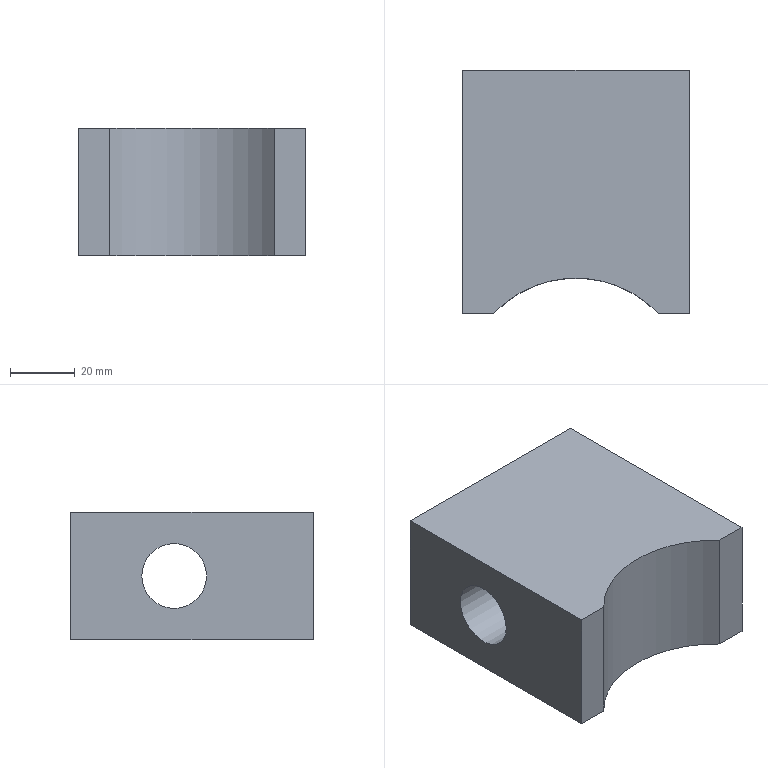Part | NX | features 推移千斤顶约束块 2 | 1 solid | 9 faces | box 70 x 75 x 39.28 mm | volume 169219 mm3 | plane 7 | cylinder 2 | commonest cylinder face diameters 20 x1 70 x1
STEP:
#1=CARTESIAN_POINT('',(0.,-42.,19.64));
#2=VERTEX_POINT('',#1);
#3=CARTESIAN_POINT('',(0.,-32.,19.64));
#4=DIRECTION('',(-1.,0.,0.));
#5=DIRECTION('',(0.,-1.,0.));
#6=AXIS2_PLACEMENT_3D('',#3,#4,#5);
#7=CIRCLE('',#6,10.);
#8=EDGE_CURVE('',#2,#2,#7,.T.);
#9=ORIENTED_EDGE('',*,*,#8,.F.);
#10=EDGE_LOOP('',(#9));
#11=FACE_BOUND('',#10,.T.);
#12=CARTESIAN_POINT('',(0.,0.,0.));
#13=VERTEX_POINT('',#12);
#14=CARTESIAN_POINT('',(0.,-75.,0.));
#15=VERTEX_POINT('',#14);
#16=CARTESIAN_POINT('',(0.,0.,0.));
#17=DIRECTION('',(0.,-1.,0.));
#18=VECTOR('',#17,1000.);
#19=LINE('',#16,#18);
#20=EDGE_CURVE('',#13,#15,#19,.T.);
#21=ORIENTED_EDGE('',*,*,#20,.T.);
#22=CARTESIAN_POINT('',(0.,-75.,39.28));
#23=VERTEX_POINT('',#22);
#24=CARTESIAN_POINT('',(0.,-75.,39.28));
#25=DIRECTION('',(0.,0.,-1.));
#26=VECTOR('',#25,1000.);
#27=LINE('',#24,#26);
#28=EDGE_CURVE('',#23,#15,#27,.T.);
#29=ORIENTED_EDGE('',*,*,#28,.F.);
#30=CARTESIAN_POINT('',(0.,0.,39.28));
#31=VERTEX_POINT('',#30);
#32=CARTESIAN_POINT('',(0.,0.,39.28));
#33=DIRECTION('',(0.,-1.,0.));
#34=VECTOR('',#33,1000.);
#35=LINE('',#32,#34);
#36=EDGE_CURVE('',#31,#23,#35,.T.);
#37=ORIENTED_EDGE('',*,*,#36,.F.);
#38=CARTESIAN_POINT('',(0.,0.,39.28));
#39=DIRECTION('',(0.,0.,-1.));
#40=VECTOR('',#39,1000.);
#41=LINE('',#38,#40);
#42=EDGE_CURVE('',#31,#13,#41,.T.);
#43=ORIENTED_EDGE('',*,*,#42,.T.);
#44=EDGE_LOOP('',(#21,#29,#37,#43));
#45=FACE_BOUND('',#44,.T.);
#46=CARTESIAN_POINT('',(0.,0.,39.28));
#47=DIRECTION('',(1.,0.,0.));
#48=DIRECTION('',(0.,1.,0.));
#49=AXIS2_PLACEMENT_3D('',#46,#47,#48);
#50=PLANE('',#49);
#51=ADVANCED_FACE('',(#11,#45),#50,.F.);
#52=CARTESIAN_POINT('',(9.619,-75.,0.));
#53=VERTEX_POINT('',#52);
#54=CARTESIAN_POINT('',(0.,-75.,0.));
#55=DIRECTION('',(1.,0.,0.));
#56=VECTOR('',#55,1000.);
#57=LINE('',#54,#56);
#58=EDGE_CURVE('',#15,#53,#57,.T.);
#59=ORIENTED_EDGE('',*,*,#58,.T.);
#60=CARTESIAN_POINT('',(9.619,-75.,39.28));
#61=VERTEX_POINT('',#60);
#62=CARTESIAN_POINT('',(9.619,-75.,39.28));
#63=DIRECTION('',(0.,0.,-1.));
#64=VECTOR('',#63,1000.);
#65=LINE('',#62,#64);
#66=EDGE_CURVE('',#61,#53,#65,.T.);
#67=ORIENTED_EDGE('',*,*,#66,.F.);
#68=CARTESIAN_POINT('',(0.,-75.,39.28));
#69=DIRECTION('',(1.,0.,0.));
#70=VECTOR('',#69,1000.);
#71=LINE('',#68,#70);
#72=EDGE_CURVE('',#23,#61,#71,.T.);
#73=ORIENTED_EDGE('',*,*,#72,.F.);
#74=ORIENTED_EDGE('',*,*,#28,.T.);
#75=EDGE_LOOP('',(#59,#67,#73,#74));
#76=FACE_BOUND('',#75,.T.);
#77=CARTESIAN_POINT('',(0.,-75.,39.28));
#78=DIRECTION('',(0.,1.,0.));
#79=DIRECTION('',(-1.,0.,0.));
#80=AXIS2_PLACEMENT_3D('',#77,#78,#79);
#81=PLANE('',#80);
#82=ADVANCED_FACE('',(#76),#81,.F.);
#83=CARTESIAN_POINT('',(60.381,-75.,0.));
#84=VERTEX_POINT('',#83);
#85=CARTESIAN_POINT('',(35.,-99.1,0.));
#86=DIRECTION('',(0.,0.,-1.));
#87=DIRECTION('',(1.,0.,0.));
#88=AXIS2_PLACEMENT_3D('',#85,#86,#87);
#89=CIRCLE('',#88,35.);
#90=EDGE_CURVE('',#53,#84,#89,.T.);
#91=ORIENTED_EDGE('',*,*,#90,.T.);
#92=CARTESIAN_POINT('',(60.381,-75.,39.28));
#93=VERTEX_POINT('',#92);
#94=CARTESIAN_POINT('',(60.381,-75.,39.28));
#95=DIRECTION('',(0.,0.,-1.));
#96=VECTOR('',#95,1000.);
#97=LINE('',#94,#96);
#98=EDGE_CURVE('',#93,#84,#97,.T.);
#99=ORIENTED_EDGE('',*,*,#98,.F.);
#100=CARTESIAN_POINT('',(35.,-99.1,39.28));
#101=DIRECTION('',(0.,0.,-1.));
#102=DIRECTION('',(1.,0.,0.));
#103=AXIS2_PLACEMENT_3D('',#100,#101,#102);
#104=CIRCLE('',#103,35.);
#105=EDGE_CURVE('',#61,#93,#104,.T.);
#106=ORIENTED_EDGE('',*,*,#105,.F.);
#107=ORIENTED_EDGE('',*,*,#66,.T.);
#108=EDGE_LOOP('',(#91,#99,#106,#107));
#109=FACE_BOUND('',#108,.T.);
#110=CARTESIAN_POINT('',(35.,-99.1,39.28));
#111=DIRECTION('',(0.,0.,-1.));
#112=DIRECTION('',(-1.,0.,0.));
#113=AXIS2_PLACEMENT_3D('',#110,#111,#112);
#114=CYLINDRICAL_SURFACE('',#113,35.);
#115=ADVANCED_FACE('',(#109),#114,.F.);
#116=CARTESIAN_POINT('',(70.,-75.,0.));
#117=VERTEX_POINT('',#116);
#118=CARTESIAN_POINT('',(60.381,-75.,0.));
#119=DIRECTION('',(1.,0.,0.));
#120=VECTOR('',#119,1000.);
#121=LINE('',#118,#120);
#122=EDGE_CURVE('',#84,#117,#121,.T.);
#123=ORIENTED_EDGE('',*,*,#122,.T.);
#124=CARTESIAN_POINT('',(70.,-75.,39.28));
#125=VERTEX_POINT('',#124);
#126=CARTESIAN_POINT('',(70.,-75.,39.28));
#127=DIRECTION('',(0.,0.,-1.));
#128=VECTOR('',#127,1000.);
#129=LINE('',#126,#128);
#130=EDGE_CURVE('',#125,#117,#129,.T.);
#131=ORIENTED_EDGE('',*,*,#130,.F.);
#132=CARTESIAN_POINT('',(60.381,-75.,39.28));
#133=DIRECTION('',(1.,0.,0.));
#134=VECTOR('',#133,1000.);
#135=LINE('',#132,#134);
#136=EDGE_CURVE('',#93,#125,#135,.T.);
#137=ORIENTED_EDGE('',*,*,#136,.F.);
#138=ORIENTED_EDGE('',*,*,#98,.T.);
#139=EDGE_LOOP('',(#123,#131,#137,#138));
#140=FACE_BOUND('',#139,.T.);
#141=CARTESIAN_POINT('',(60.381,-75.,39.28));
#142=DIRECTION('',(0.,1.,0.));
#143=DIRECTION('',(0.,0.,1.));
#144=AXIS2_PLACEMENT_3D('',#141,#142,#143);
#145=PLANE('',#144);
#146=ADVANCED_FACE('',(#140),#145,.F.);
#147=CARTESIAN_POINT('',(70.,-42.,19.64));
#148=VERTEX_POINT('',#147);
#149=CARTESIAN_POINT('',(70.,-32.,19.64));
#150=DIRECTION('',(-1.,0.,0.));
#151=DIRECTION('',(0.,-1.,0.));
#152=AXIS2_PLACEMENT_3D('',#149,#150,#151);
#153=CIRCLE('',#152,10.);
#154=EDGE_CURVE('',#148,#148,#153,.T.);
#155=ORIENTED_EDGE('',*,*,#154,.T.);
#156=EDGE_LOOP('',(#155));
#157=FACE_BOUND('',#156,.T.);
#158=CARTESIAN_POINT('',(70.,0.,0.));
#159=VERTEX_POINT('',#158);
#160=CARTESIAN_POINT('',(70.,0.,0.));
#161=DIRECTION('',(0.,1.,0.));
#162=VECTOR('',#161,1000.);
#163=LINE('',#160,#162);
#164=EDGE_CURVE('',#117,#159,#163,.T.);
#165=ORIENTED_EDGE('',*,*,#164,.T.);
#166=CARTESIAN_POINT('',(70.,0.,39.28));
#167=VERTEX_POINT('',#166);
#168=CARTESIAN_POINT('',(70.,0.,39.28));
#169=DIRECTION('',(0.,0.,-1.));
#170=VECTOR('',#169,1000.);
#171=LINE('',#168,#170);
#172=EDGE_CURVE('',#167,#159,#171,.T.);
#173=ORIENTED_EDGE('',*,*,#172,.F.);
#174=CARTESIAN_POINT('',(70.,0.,39.28));
#175=DIRECTION('',(0.,1.,0.));
#176=VECTOR('',#175,1000.);
#177=LINE('',#174,#176);
#178=EDGE_CURVE('',#125,#167,#177,.T.);
#179=ORIENTED_EDGE('',*,*,#178,.F.);
#180=ORIENTED_EDGE('',*,*,#130,.T.);
#181=EDGE_LOOP('',(#165,#173,#179,#180));
#182=FACE_BOUND('',#181,.T.);
#183=CARTESIAN_POINT('',(70.,0.,39.28));
#184=DIRECTION('',(-1.,0.,0.));
#185=DIRECTION('',(0.,-1.,0.));
#186=AXIS2_PLACEMENT_3D('',#183,#184,#185);
#187=PLANE('',#186);
#188=ADVANCED_FACE('',(#157,#182),#187,.F.);
#189=CARTESIAN_POINT('',(0.,0.,0.));
#190=DIRECTION('',(-1.,0.,0.));
#191=VECTOR('',#190,1000.);
#192=LINE('',#189,#191);
#193=EDGE_CURVE('',#159,#13,#192,.T.);
#194=ORIENTED_EDGE('',*,*,#193,.T.);
#195=ORIENTED_EDGE('',*,*,#42,.F.);
#196=CARTESIAN_POINT('',(0.,0.,39.28));
#197=DIRECTION('',(-1.,0.,0.));
#198=VECTOR('',#197,1000.);
#199=LINE('',#196,#198);
#200=EDGE_CURVE('',#167,#31,#199,.T.);
#201=ORIENTED_EDGE('',*,*,#200,.F.);
#202=ORIENTED_EDGE('',*,*,#172,.T.);
#203=EDGE_LOOP('',(#194,#195,#201,#202));
#204=FACE_BOUND('',#203,.T.);
#205=CARTESIAN_POINT('',(0.,0.,39.28));
#206=DIRECTION('',(0.,-1.,0.));
#207=DIRECTION('',(0.,0.,-1.));
#208=AXIS2_PLACEMENT_3D('',#205,#206,#207);
#209=PLANE('',#208);
#210=ADVANCED_FACE('',(#204),#209,.F.);
#211=ORIENTED_EDGE('',*,*,#36,.T.);
#212=ORIENTED_EDGE('',*,*,#72,.T.);
#213=ORIENTED_EDGE('',*,*,#105,.T.);
#214=ORIENTED_EDGE('',*,*,#136,.T.);
#215=ORIENTED_EDGE('',*,*,#178,.T.);
#216=ORIENTED_EDGE('',*,*,#200,.T.);
#217=EDGE_LOOP('',(#211,#212,#213,#214,#215,#216));
#218=FACE_BOUND('',#217,.T.);
#219=CARTESIAN_POINT('',(35.,-99.1,39.28));
#220=DIRECTION('',(0.,0.,1.));
#221=DIRECTION('',(1.,0.,0.));
#222=AXIS2_PLACEMENT_3D('',#219,#220,#221);
#223=PLANE('',#222);
#224=ADVANCED_FACE('',(#218),#223,.T.);
#225=ORIENTED_EDGE('',*,*,#20,.F.);
#226=ORIENTED_EDGE('',*,*,#193,.F.);
#227=ORIENTED_EDGE('',*,*,#164,.F.);
#228=ORIENTED_EDGE('',*,*,#122,.F.);
#229=ORIENTED_EDGE('',*,*,#90,.F.);
#230=ORIENTED_EDGE('',*,*,#58,.F.);
#231=EDGE_LOOP('',(#225,#226,#227,#228,#229,#230));
#232=FACE_BOUND('',#231,.T.);
#233=CARTESIAN_POINT('',(35.,-99.1,0.));
#234=DIRECTION('',(0.,0.,1.));
#235=DIRECTION('',(1.,0.,0.));
#236=AXIS2_PLACEMENT_3D('',#233,#234,#235);
#237=PLANE('',#236);
#238=ADVANCED_FACE('',(#232),#237,.F.);
#239=ORIENTED_EDGE('',*,*,#154,.F.);
#240=EDGE_LOOP('',(#239));
#241=FACE_BOUND('',#240,.T.);
#242=ORIENTED_EDGE('',*,*,#8,.T.);
#243=EDGE_LOOP('',(#242));
#244=FACE_BOUND('',#243,.T.);
#245=CARTESIAN_POINT('',(70.,-32.,19.64));
#246=DIRECTION('',(-1.,0.,0.));
#247=DIRECTION('',(0.,-1.,0.));
#248=AXIS2_PLACEMENT_3D('',#245,#246,#247);
#249=CYLINDRICAL_SURFACE('',#248,10.);
#250=ADVANCED_FACE('',(#241,#244),#249,.F.);
#251=CLOSED_SHELL('',(#51,#82,#115,#146,#188,#210,#224,#238,#250));
#252=MANIFOLD_SOLID_BREP('',#251);
#253=(LENGTH_UNIT()NAMED_UNIT(*)SI_UNIT(.MILLI.,.METRE.));
#254=UNCERTAINTY_MEASURE_WITH_UNIT(LENGTH_MEASURE(0.00001),#253,'','');
#255=(NAMED_UNIT(*)PLANE_ANGLE_UNIT()SI_UNIT($,.RADIAN.));
#256=(NAMED_UNIT(*)SI_UNIT($,.STERADIAN.)SOLID_ANGLE_UNIT());
#257=(GEOMETRIC_REPRESENTATION_CONTEXT(3)GLOBAL_UNCERTAINTY_ASSIGNED_CONTEXT((#254))GLOBAL_UNIT_ASSIGNED_CONTEXT((#253,#255,#256))REPRESENTATION_CONTEXT('',''));
#258=ADVANCED_BREP_SHAPE_REPRESENTATION('',(#252),#257);